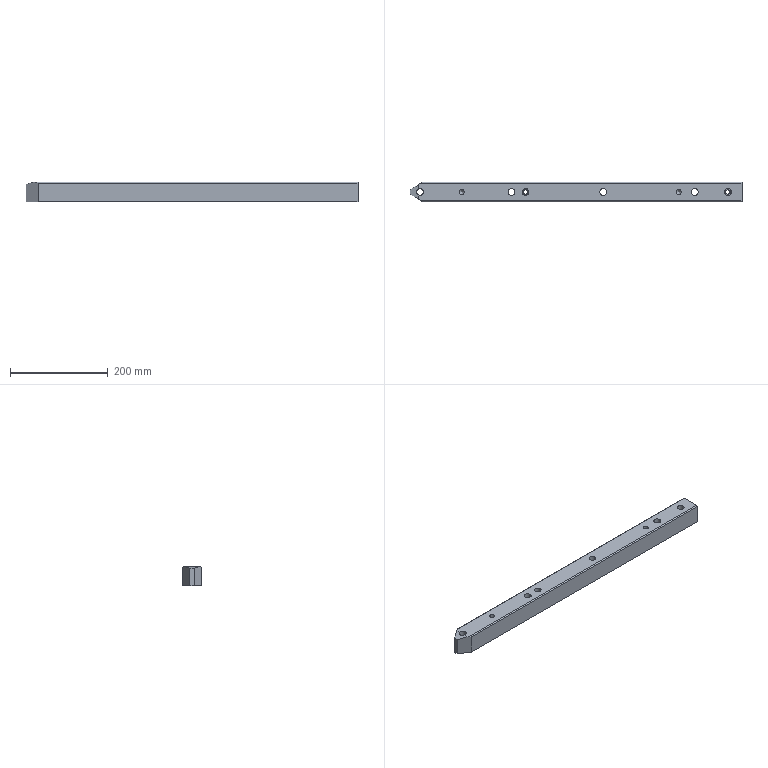Part | NX | features 22 2 | 1 solid | 35 faces | box 681 x 40 x 40 mm | volume 1019964 mm3 | plane 17 | cylinder 16 | cone 2 | commonest cylinder face diameters 14 x6 6 x4 9 x2 10.3 x2 25 x2
STEP:
#1=CARTESIAN_POINT('',(1685.15,0.,-3.5));
#2=VERTEX_POINT('',#1);
#3=CARTESIAN_POINT('',(1680.,0.,-3.5));
#4=DIRECTION('',(0.,0.,-1.));
#5=DIRECTION('',(1.,0.,0.));
#6=AXIS2_PLACEMENT_3D('',#3,#4,#5);
#7=CIRCLE('',#6,5.15);
#8=EDGE_CURVE('',#2,#2,#7,.T.);
#9=ORIENTED_EDGE('',*,*,#8,.T.);
#10=EDGE_LOOP('',(#9));
#11=FACE_BOUND('',#10,.T.);
#12=CARTESIAN_POINT('',(1344.306,0.,-3.5));
#13=VERTEX_POINT('',#12);
#14=CARTESIAN_POINT('',(1337.306,0.,-3.5));
#15=DIRECTION('',(0.,0.,-1.));
#16=DIRECTION('',(1.,0.,0.));
#17=AXIS2_PLACEMENT_3D('',#14,#15,#16);
#18=CIRCLE('',#17,7.);
#19=EDGE_CURVE('',#13,#13,#18,.T.);
#20=ORIENTED_EDGE('',*,*,#19,.T.);
#21=EDGE_LOOP('',(#20));
#22=FACE_BOUND('',#21,.T.);
#23=CARTESIAN_POINT('',(1372.578,2.394,-3.5));
#24=VERTEX_POINT('',#23);
#25=CARTESIAN_POINT('',(1366.,0.,-3.5));
#26=DIRECTION('',(0.,0.,-1.));
#27=DIRECTION('',(0.9397,0.342,0.));
#28=AXIS2_PLACEMENT_3D('',#25,#26,#27);
#29=CIRCLE('',#28,7.);
#30=EDGE_CURVE('',#24,#24,#29,.T.);
#31=ORIENTED_EDGE('',*,*,#30,.T.);
#32=EDGE_LOOP('',(#31));
#33=FACE_BOUND('',#32,.T.);
#34=CARTESIAN_POINT('',(1787.578,2.394,-3.5));
#35=VERTEX_POINT('',#34);
#36=CARTESIAN_POINT('',(1781.,0.,-3.5));
#37=DIRECTION('',(0.,0.,-1.));
#38=DIRECTION('',(0.9397,0.342,0.));
#39=AXIS2_PLACEMENT_3D('',#36,#37,#38);
#40=CIRCLE('',#39,7.);
#41=EDGE_CURVE('',#35,#35,#40,.T.);
#42=ORIENTED_EDGE('',*,*,#41,.T.);
#43=EDGE_LOOP('',(#42));
#44=FACE_BOUND('',#43,.T.);
#45=CARTESIAN_POINT('',(1146.,6.17,-3.5));
#46=VERTEX_POINT('',#45);
#47=CARTESIAN_POINT('',(1146.,-6.17,-3.5));
#48=VERTEX_POINT('',#47);
#49=CARTESIAN_POINT('',(1149.306,0.,-3.5));
#50=DIRECTION('',(0.,0.,-1.));
#51=DIRECTION('',(1.,0.,0.));
#52=AXIS2_PLACEMENT_3D('',#49,#50,#51);
#53=CIRCLE('',#52,7.);
#54=EDGE_CURVE('',#46,#48,#53,.T.);
#55=ORIENTED_EDGE('',*,*,#54,.T.);
#56=CARTESIAN_POINT('',(1146.,-14.83,-3.5));
#57=VERTEX_POINT('',#56);
#58=CARTESIAN_POINT('',(1146.,0.,-3.5));
#59=DIRECTION('',(0.,-1.,0.));
#60=VECTOR('',#59,1000.);
#61=LINE('',#58,#60);
#62=EDGE_CURVE('',#48,#57,#61,.T.);
#63=ORIENTED_EDGE('',*,*,#62,.T.);
#64=CARTESIAN_POINT('',(1151.084,-18.,-3.5));
#65=VERTEX_POINT('',#64);
#66=CARTESIAN_POINT('',(921.823,124.98,-3.5));
#67=DIRECTION('',(0.8485,-0.5292,0.));
#68=VECTOR('',#67,1000.);
#69=LINE('',#66,#68);
#70=EDGE_CURVE('',#57,#65,#69,.T.);
#71=ORIENTED_EDGE('',*,*,#70,.T.);
#72=CARTESIAN_POINT('',(1810.,-18.,-3.5));
#73=VERTEX_POINT('',#72);
#74=CARTESIAN_POINT('',(883.879,-18.,-3.5));
#75=DIRECTION('',(1.,0.,0.));
#76=VECTOR('',#75,1000.);
#77=LINE('',#74,#76);
#78=EDGE_CURVE('',#65,#73,#77,.T.);
#79=ORIENTED_EDGE('',*,*,#78,.T.);
#80=CARTESIAN_POINT('',(1810.,18.,-3.5));
#81=VERTEX_POINT('',#80);
#82=CARTESIAN_POINT('',(1810.,0.,-3.5));
#83=DIRECTION('',(0.,1.,0.));
#84=VECTOR('',#83,1000.);
#85=LINE('',#82,#84);
#86=EDGE_CURVE('',#73,#81,#85,.T.);
#87=ORIENTED_EDGE('',*,*,#86,.T.);
#88=CARTESIAN_POINT('',(1151.084,18.,-3.5));
#89=VERTEX_POINT('',#88);
#90=CARTESIAN_POINT('',(883.879,18.,-3.5));
#91=DIRECTION('',(-1.,0.,0.));
#92=VECTOR('',#91,1000.);
#93=LINE('',#90,#92);
#94=EDGE_CURVE('',#81,#89,#93,.T.);
#95=ORIENTED_EDGE('',*,*,#94,.T.);
#96=CARTESIAN_POINT('',(1146.,14.83,-3.5));
#97=VERTEX_POINT('',#96);
#98=CARTESIAN_POINT('',(1130.298,5.037,-3.5));
#99=DIRECTION('',(0.8485,0.5292,0.));
#100=VECTOR('',#99,1000.);
#101=LINE('',#98,#100);
#102=EDGE_CURVE('',#97,#89,#101,.T.);
#103=ORIENTED_EDGE('',*,*,#102,.F.);
#104=CARTESIAN_POINT('',(1146.,0.,-3.5));
#105=DIRECTION('',(0.,-1.,0.));
#106=VECTOR('',#105,1000.);
#107=LINE('',#104,#106);
#108=EDGE_CURVE('',#97,#46,#107,.T.);
#109=ORIENTED_EDGE('',*,*,#108,.T.);
#110=EDGE_LOOP('',(#55,#63,#71,#79,#87,#95,#103,#109));
#111=FACE_BOUND('',#110,.T.);
#112=CARTESIAN_POINT('',(1532.306,0.,-3.5));
#113=VERTEX_POINT('',#112);
#114=CARTESIAN_POINT('',(1525.306,0.,-3.5));
#115=DIRECTION('',(0.,0.,1.));
#116=DIRECTION('',(1.,0.,0.));
#117=AXIS2_PLACEMENT_3D('',#114,#115,#116);
#118=CIRCLE('',#117,7.);
#119=EDGE_CURVE('',#113,#113,#118,.T.);
#120=ORIENTED_EDGE('',*,*,#119,.F.);
#121=EDGE_LOOP('',(#120));
#122=FACE_BOUND('',#121,.T.);
#123=CARTESIAN_POINT('',(1720.306,0.,-3.5));
#124=VERTEX_POINT('',#123);
#125=CARTESIAN_POINT('',(1713.306,0.,-3.5));
#126=DIRECTION('',(0.,0.,1.));
#127=DIRECTION('',(1.,0.,0.));
#128=AXIS2_PLACEMENT_3D('',#125,#126,#127);
#129=CIRCLE('',#128,7.);
#130=EDGE_CURVE('',#124,#124,#129,.T.);
#131=ORIENTED_EDGE('',*,*,#130,.F.);
#132=EDGE_LOOP('',(#131));
#133=FACE_BOUND('',#132,.T.);
#134=CARTESIAN_POINT('',(1240.15,0.,-3.5));
#135=VERTEX_POINT('',#134);
#136=CARTESIAN_POINT('',(1235.,0.,-3.5));
#137=DIRECTION('',(0.,0.,-1.));
#138=DIRECTION('',(1.,0.,0.));
#139=AXIS2_PLACEMENT_3D('',#136,#137,#138);
#140=CIRCLE('',#139,5.15);
#141=EDGE_CURVE('',#135,#135,#140,.T.);
#142=ORIENTED_EDGE('',*,*,#141,.T.);
#143=EDGE_LOOP('',(#142));
#144=FACE_BOUND('',#143,.T.);
#145=CARTESIAN_POINT('',(883.879,0.,-3.5));
#146=DIRECTION('',(0.,0.,1.));
#147=DIRECTION('',(-1.,0.,0.));
#148=AXIS2_PLACEMENT_3D('',#145,#146,#147);
#149=PLANE('',#148);
#150=ADVANCED_FACE('',(#11,#22,#33,#44,#111,#122,#133,#144),#149,.T.);
#151=CARTESIAN_POINT('',(1344.306,0.,-43.5));
#152=VERTEX_POINT('',#151);
#153=CARTESIAN_POINT('',(1337.306,0.,-43.5));
#154=DIRECTION('',(0.,0.,-1.));
#155=DIRECTION('',(1.,0.,0.));
#156=AXIS2_PLACEMENT_3D('',#153,#154,#155);
#157=CIRCLE('',#156,7.);
#158=EDGE_CURVE('',#152,#152,#157,.T.);
#159=ORIENTED_EDGE('',*,*,#158,.F.);
#160=EDGE_LOOP('',(#159));
#161=FACE_BOUND('',#160,.T.);
#162=CARTESIAN_POINT('',(1810.,20.,-43.5));
#163=VERTEX_POINT('',#162);
#164=CARTESIAN_POINT('',(1154.291,20.,-43.5));
#165=VERTEX_POINT('',#164);
#166=CARTESIAN_POINT('',(1199.,20.,-43.5));
#167=DIRECTION('',(-1.,0.,0.));
#168=VECTOR('',#167,1000.);
#169=LINE('',#166,#168);
#170=EDGE_CURVE('',#163,#165,#169,.T.);
#171=ORIENTED_EDGE('',*,*,#170,.F.);
#172=CARTESIAN_POINT('',(1810.,-20.,-43.5));
#173=VERTEX_POINT('',#172);
#174=CARTESIAN_POINT('',(1810.,0.,-43.5));
#175=DIRECTION('',(0.,-1.,0.));
#176=VECTOR('',#175,1000.);
#177=LINE('',#174,#176);
#178=EDGE_CURVE('',#163,#173,#177,.T.);
#179=ORIENTED_EDGE('',*,*,#178,.T.);
#180=CARTESIAN_POINT('',(1154.291,-20.,-43.5));
#181=VERTEX_POINT('',#180);
#182=CARTESIAN_POINT('',(1199.,-20.,-43.5));
#183=DIRECTION('',(1.,0.,0.));
#184=VECTOR('',#183,1000.);
#185=LINE('',#182,#184);
#186=EDGE_CURVE('',#181,#173,#185,.T.);
#187=ORIENTED_EDGE('',*,*,#186,.F.);
#188=CARTESIAN_POINT('',(1129.,-4.227,-43.5));
#189=VERTEX_POINT('',#188);
#190=CARTESIAN_POINT('',(921.823,124.98,-43.5));
#191=DIRECTION('',(-0.8485,0.5292,0.));
#192=VECTOR('',#191,1000.);
#193=LINE('',#190,#192);
#194=EDGE_CURVE('',#181,#189,#193,.T.);
#195=ORIENTED_EDGE('',*,*,#194,.T.);
#196=CARTESIAN_POINT('',(1129.,4.227,-43.5));
#197=VERTEX_POINT('',#196);
#198=CARTESIAN_POINT('',(1129.,0.,-43.5));
#199=DIRECTION('',(0.,-1.,0.));
#200=VECTOR('',#199,1000.);
#201=LINE('',#198,#200);
#202=EDGE_CURVE('',#197,#189,#201,.T.);
#203=ORIENTED_EDGE('',*,*,#202,.F.);
#204=CARTESIAN_POINT('',(921.823,-124.98,-43.5));
#205=DIRECTION('',(0.8485,0.5292,0.));
#206=VECTOR('',#205,1000.);
#207=LINE('',#204,#206);
#208=EDGE_CURVE('',#197,#165,#207,.T.);
#209=ORIENTED_EDGE('',*,*,#208,.T.);
#210=EDGE_LOOP('',(#171,#179,#187,#195,#203,#209));
#211=FACE_BOUND('',#210,.T.);
#212=CARTESIAN_POINT('',(1783.701,-11.,-43.5));
#213=VERTEX_POINT('',#212);
#214=CARTESIAN_POINT('',(1778.299,-11.,-43.5));
#215=VERTEX_POINT('',#214);
#216=CARTESIAN_POINT('',(1781.,-11.,-43.5));
#217=DIRECTION('',(-1.,0.,0.));
#218=VECTOR('',#217,1000.);
#219=LINE('',#216,#218);
#220=EDGE_CURVE('',#213,#215,#219,.T.);
#221=ORIENTED_EDGE('',*,*,#220,.F.);
#222=CARTESIAN_POINT('',(1788.847,-9.73,-43.5));
#223=VERTEX_POINT('',#222);
#224=CARTESIAN_POINT('',(1785.937,-9.,-43.5));
#225=DIRECTION('',(0.,0.,-1.));
#226=DIRECTION('',(1.,0.,0.));
#227=AXIS2_PLACEMENT_3D('',#224,#225,#226);
#228=CIRCLE('',#227,3.);
#229=EDGE_CURVE('',#223,#213,#228,.T.);
#230=ORIENTED_EDGE('',*,*,#229,.F.);
#231=CARTESIAN_POINT('',(1773.153,-9.73,-43.5));
#232=VERTEX_POINT('',#231);
#233=CARTESIAN_POINT('',(1781.,0.,-43.5));
#234=DIRECTION('',(0.,0.,-1.));
#235=DIRECTION('',(1.,0.,0.));
#236=AXIS2_PLACEMENT_3D('',#233,#234,#235);
#237=CIRCLE('',#236,12.5);
#238=EDGE_CURVE('',#232,#223,#237,.T.);
#239=ORIENTED_EDGE('',*,*,#238,.F.);
#240=CARTESIAN_POINT('',(1776.063,-9.,-43.5));
#241=DIRECTION('',(0.,0.,-1.));
#242=DIRECTION('',(1.,0.,0.));
#243=AXIS2_PLACEMENT_3D('',#240,#241,#242);
#244=CIRCLE('',#243,3.);
#245=EDGE_CURVE('',#215,#232,#244,.T.);
#246=ORIENTED_EDGE('',*,*,#245,.F.);
#247=EDGE_LOOP('',(#221,#230,#239,#246));
#248=FACE_BOUND('',#247,.T.);
#249=CARTESIAN_POINT('',(1368.701,-11.,-43.5));
#250=VERTEX_POINT('',#249);
#251=CARTESIAN_POINT('',(1363.299,-11.,-43.5));
#252=VERTEX_POINT('',#251);
#253=CARTESIAN_POINT('',(1366.,-11.,-43.5));
#254=DIRECTION('',(-1.,0.,0.));
#255=VECTOR('',#254,1000.);
#256=LINE('',#253,#255);
#257=EDGE_CURVE('',#250,#252,#256,.T.);
#258=ORIENTED_EDGE('',*,*,#257,.F.);
#259=CARTESIAN_POINT('',(1373.847,-9.73,-43.5));
#260=VERTEX_POINT('',#259);
#261=CARTESIAN_POINT('',(1370.937,-9.,-43.5));
#262=DIRECTION('',(0.,0.,-1.));
#263=DIRECTION('',(0.9659,0.2588,0.));
#264=AXIS2_PLACEMENT_3D('',#261,#262,#263);
#265=CIRCLE('',#264,3.);
#266=EDGE_CURVE('',#260,#250,#265,.T.);
#267=ORIENTED_EDGE('',*,*,#266,.F.);
#268=CARTESIAN_POINT('',(1358.153,-9.73,-43.5));
#269=VERTEX_POINT('',#268);
#270=CARTESIAN_POINT('',(1366.,0.,-43.5));
#271=DIRECTION('',(0.,0.,1.));
#272=DIRECTION('',(0.9659,0.2588,0.));
#273=AXIS2_PLACEMENT_3D('',#270,#271,#272);
#274=CIRCLE('',#273,12.5);
#275=EDGE_CURVE('',#260,#269,#274,.T.);
#276=ORIENTED_EDGE('',*,*,#275,.T.);
#277=CARTESIAN_POINT('',(1361.063,-9.,-43.5));
#278=DIRECTION('',(0.,0.,-1.));
#279=DIRECTION('',(0.9659,0.2588,0.));
#280=AXIS2_PLACEMENT_3D('',#277,#278,#279);
#281=CIRCLE('',#280,3.);
#282=EDGE_CURVE('',#252,#269,#281,.T.);
#283=ORIENTED_EDGE('',*,*,#282,.F.);
#284=EDGE_LOOP('',(#258,#267,#276,#283));
#285=FACE_BOUND('',#284,.T.);
#286=CARTESIAN_POINT('',(1156.306,0.,-43.5));
#287=VERTEX_POINT('',#286);
#288=CARTESIAN_POINT('',(1149.306,0.,-43.5));
#289=DIRECTION('',(0.,0.,1.));
#290=DIRECTION('',(1.,0.,0.));
#291=AXIS2_PLACEMENT_3D('',#288,#289,#290);
#292=CIRCLE('',#291,7.);
#293=EDGE_CURVE('',#287,#287,#292,.T.);
#294=ORIENTED_EDGE('',*,*,#293,.T.);
#295=EDGE_LOOP('',(#294));
#296=FACE_BOUND('',#295,.T.);
#297=CARTESIAN_POINT('',(1532.306,0.,-43.5));
#298=VERTEX_POINT('',#297);
#299=CARTESIAN_POINT('',(1525.306,0.,-43.5));
#300=DIRECTION('',(0.,0.,1.));
#301=DIRECTION('',(1.,0.,0.));
#302=AXIS2_PLACEMENT_3D('',#299,#300,#301);
#303=CIRCLE('',#302,7.);
#304=EDGE_CURVE('',#298,#298,#303,.T.);
#305=ORIENTED_EDGE('',*,*,#304,.T.);
#306=EDGE_LOOP('',(#305));
#307=FACE_BOUND('',#306,.T.);
#308=CARTESIAN_POINT('',(1720.306,0.,-43.5));
#309=VERTEX_POINT('',#308);
#310=CARTESIAN_POINT('',(1713.306,0.,-43.5));
#311=DIRECTION('',(0.,0.,-1.));
#312=DIRECTION('',(1.,0.,0.));
#313=AXIS2_PLACEMENT_3D('',#310,#311,#312);
#314=CIRCLE('',#313,7.);
#315=EDGE_CURVE('',#309,#309,#314,.T.);
#316=ORIENTED_EDGE('',*,*,#315,.F.);
#317=EDGE_LOOP('',(#316));
#318=FACE_BOUND('',#317,.T.);
#319=CARTESIAN_POINT('',(883.879,0.,-43.5));
#320=DIRECTION('',(0.,0.,1.));
#321=DIRECTION('',(-1.,0.,0.));
#322=AXIS2_PLACEMENT_3D('',#319,#320,#321);
#323=PLANE('',#322);
#324=ADVANCED_FACE('',(#161,#211,#248,#285,#296,#307,#318),#323,.F.);
#325=CARTESIAN_POINT('',(1154.291,20.,-5.5));
#326=VERTEX_POINT('',#325);
#327=CARTESIAN_POINT('',(1810.,20.,-5.5));
#328=VERTEX_POINT('',#327);
#329=CARTESIAN_POINT('',(1199.,20.,-5.5));
#330=DIRECTION('',(1.,0.,0.));
#331=VECTOR('',#330,1000.);
#332=LINE('',#329,#331);
#333=EDGE_CURVE('',#326,#328,#332,.T.);
#334=ORIENTED_EDGE('',*,*,#333,.T.);
#335=CARTESIAN_POINT('',(1810.,20.,-23.5));
#336=DIRECTION('',(0.,0.,-1.));
#337=VECTOR('',#336,1000.);
#338=LINE('',#335,#337);
#339=EDGE_CURVE('',#328,#163,#338,.T.);
#340=ORIENTED_EDGE('',*,*,#339,.T.);
#341=ORIENTED_EDGE('',*,*,#170,.T.);
#342=CARTESIAN_POINT('',(1154.291,20.,-23.5));
#343=DIRECTION('',(0.,0.,1.));
#344=VECTOR('',#343,1000.);
#345=LINE('',#342,#344);
#346=EDGE_CURVE('',#165,#326,#345,.T.);
#347=ORIENTED_EDGE('',*,*,#346,.T.);
#348=EDGE_LOOP('',(#334,#340,#341,#347));
#349=FACE_BOUND('',#348,.T.);
#350=CARTESIAN_POINT('',(1199.,20.,-23.5));
#351=DIRECTION('',(0.,1.,0.));
#352=DIRECTION('',(0.,0.,-1.));
#353=AXIS2_PLACEMENT_3D('',#350,#351,#352);
#354=PLANE('',#353);
#355=ADVANCED_FACE('',(#349),#354,.T.);
#356=ORIENTED_EDGE('',*,*,#94,.F.);
#357=CARTESIAN_POINT('',(1810.,18.,-3.5));
#358=DIRECTION('',(0.,0.7071,-0.7071));
#359=VECTOR('',#358,1000.);
#360=LINE('',#357,#359);
#361=EDGE_CURVE('',#81,#328,#360,.T.);
#362=ORIENTED_EDGE('',*,*,#361,.T.);
#363=ORIENTED_EDGE('',*,*,#333,.F.);
#364=CARTESIAN_POINT('',(978.292,-89.762,104.262));
#365=DIRECTION('',(-0.75,-0.4677,0.4677));
#366=VECTOR('',#365,1000.);
#367=LINE('',#364,#366);
#368=EDGE_CURVE('',#326,#89,#367,.T.);
#369=ORIENTED_EDGE('',*,*,#368,.T.);
#370=EDGE_LOOP('',(#356,#362,#363,#369));
#371=FACE_BOUND('',#370,.T.);
#372=CARTESIAN_POINT('',(883.879,18.,-3.5));
#373=DIRECTION('',(0.,-0.7071,-0.7071));
#374=DIRECTION('',(0.,-0.7071,0.7071));
#375=AXIS2_PLACEMENT_3D('',#372,#373,#374);
#376=PLANE('',#375);
#377=ADVANCED_FACE('',(#371),#376,.F.);
#378=ORIENTED_EDGE('',*,*,#186,.T.);
#379=CARTESIAN_POINT('',(1810.,-20.,-5.5));
#380=VERTEX_POINT('',#379);
#381=CARTESIAN_POINT('',(1810.,-20.,-23.5));
#382=DIRECTION('',(0.,0.,1.));
#383=VECTOR('',#382,1000.);
#384=LINE('',#381,#383);
#385=EDGE_CURVE('',#173,#380,#384,.T.);
#386=ORIENTED_EDGE('',*,*,#385,.T.);
#387=CARTESIAN_POINT('',(1154.291,-20.,-5.5));
#388=VERTEX_POINT('',#387);
#389=CARTESIAN_POINT('',(1199.,-20.,-5.5));
#390=DIRECTION('',(-1.,0.,0.));
#391=VECTOR('',#390,1000.);
#392=LINE('',#389,#391);
#393=EDGE_CURVE('',#380,#388,#392,.T.);
#394=ORIENTED_EDGE('',*,*,#393,.T.);
#395=CARTESIAN_POINT('',(1154.291,-20.,-23.5));
#396=DIRECTION('',(0.,0.,-1.));
#397=VECTOR('',#396,1000.);
#398=LINE('',#395,#397);
#399=EDGE_CURVE('',#388,#181,#398,.T.);
#400=ORIENTED_EDGE('',*,*,#399,.T.);
#401=EDGE_LOOP('',(#378,#386,#394,#400));
#402=FACE_BOUND('',#401,.T.);
#403=CARTESIAN_POINT('',(1199.,-20.,-23.5));
#404=DIRECTION('',(0.,-1.,0.));
#405=DIRECTION('',(0.,0.,1.));
#406=AXIS2_PLACEMENT_3D('',#403,#404,#405);
#407=PLANE('',#406);
#408=ADVANCED_FACE('',(#402),#407,.T.);
#409=ORIENTED_EDGE('',*,*,#393,.F.);
#410=CARTESIAN_POINT('',(1810.,-18.,-3.5));
#411=DIRECTION('',(0.,0.7071,0.7071));
#412=VECTOR('',#411,1000.);
#413=LINE('',#410,#412);
#414=EDGE_CURVE('',#380,#73,#413,.T.);
#415=ORIENTED_EDGE('',*,*,#414,.T.);
#416=ORIENTED_EDGE('',*,*,#78,.F.);
#417=CARTESIAN_POINT('',(978.292,89.762,104.262));
#418=DIRECTION('',(0.75,-0.4677,-0.4677));
#419=VECTOR('',#418,1000.);
#420=LINE('',#417,#419);
#421=EDGE_CURVE('',#65,#388,#420,.T.);
#422=ORIENTED_EDGE('',*,*,#421,.T.);
#423=EDGE_LOOP('',(#409,#415,#416,#422));
#424=FACE_BOUND('',#423,.T.);
#425=CARTESIAN_POINT('',(883.879,-18.,-3.5));
#426=DIRECTION('',(0.,0.7071,-0.7071));
#427=DIRECTION('',(0.,-0.7071,-0.7071));
#428=AXIS2_PLACEMENT_3D('',#425,#426,#427);
#429=PLANE('',#428);
#430=ADVANCED_FACE('',(#424),#429,.F.);
#431=CARTESIAN_POINT('',(1129.,-4.227,-7.75));
#432=VERTEX_POINT('',#431);
#433=CARTESIAN_POINT('',(1124.987,-1.725,-8.753));
#434=DIRECTION('',(0.83,-0.5177,0.2075));
#435=VECTOR('',#434,1000.);
#436=LINE('',#433,#435);
#437=EDGE_CURVE('',#432,#57,#436,.T.);
#438=ORIENTED_EDGE('',*,*,#437,.F.);
#439=CARTESIAN_POINT('',(1129.,-4.227,-23.5));
#440=DIRECTION('',(0.,0.,1.));
#441=VECTOR('',#440,1000.);
#442=LINE('',#439,#441);
#443=EDGE_CURVE('',#189,#432,#442,.T.);
#444=ORIENTED_EDGE('',*,*,#443,.F.);
#445=ORIENTED_EDGE('',*,*,#194,.F.);
#446=ORIENTED_EDGE('',*,*,#399,.F.);
#447=ORIENTED_EDGE('',*,*,#421,.F.);
#448=ORIENTED_EDGE('',*,*,#70,.F.);
#449=EDGE_LOOP('',(#438,#444,#445,#446,#447,#448));
#450=FACE_BOUND('',#449,.T.);
#451=CARTESIAN_POINT('',(1130.298,-5.037,-13.5));
#452=DIRECTION('',(-0.5292,-0.8485,0.));
#453=DIRECTION('',(0.8485,-0.5292,0.));
#454=AXIS2_PLACEMENT_3D('',#451,#452,#453);
#455=PLANE('',#454);
#456=ADVANCED_FACE('',(#450),#455,.T.);
#457=CARTESIAN_POINT('',(1781.,-4.5,-28.5));
#458=VERTEX_POINT('',#457);
#459=CARTESIAN_POINT('',(1781.,0.,-28.5));
#460=DIRECTION('',(0.,0.,1.));
#461=DIRECTION('',(0.,-1.,0.));
#462=AXIS2_PLACEMENT_3D('',#459,#460,#461);
#463=CIRCLE('',#462,4.5);
#464=EDGE_CURVE('',#458,#458,#463,.T.);
#465=ORIENTED_EDGE('',*,*,#464,.F.);
#466=EDGE_LOOP('',(#465));
#467=FACE_BOUND('',#466,.T.);
#468=CARTESIAN_POINT('',(1781.,-4.5,-15.5));
#469=VERTEX_POINT('',#468);
#470=CARTESIAN_POINT('',(1781.,0.,-15.5));
#471=DIRECTION('',(0.,0.,1.));
#472=DIRECTION('',(0.,-1.,0.));
#473=AXIS2_PLACEMENT_3D('',#470,#471,#472);
#474=CIRCLE('',#473,4.5);
#475=EDGE_CURVE('',#469,#469,#474,.T.);
#476=ORIENTED_EDGE('',*,*,#475,.T.);
#477=EDGE_LOOP('',(#476));
#478=FACE_BOUND('',#477,.T.);
#479=CARTESIAN_POINT('',(1781.,0.,49.9));
#480=DIRECTION('',(0.,0.,-1.));
#481=DIRECTION('',(0.342,-0.9397,0.));
#482=AXIS2_PLACEMENT_3D('',#479,#480,#481);
#483=CYLINDRICAL_SURFACE('',#482,4.5);
#484=ADVANCED_FACE('',(#467,#478),#483,.F.);
#485=CARTESIAN_POINT('',(1370.229,1.539,-28.5));
#486=VERTEX_POINT('',#485);
#487=CARTESIAN_POINT('',(1366.,0.,-28.5));
#488=DIRECTION('',(0.,0.,1.));
#489=DIRECTION('',(0.9397,0.342,0.));
#490=AXIS2_PLACEMENT_3D('',#487,#488,#489);
#491=CIRCLE('',#490,4.5);
#492=EDGE_CURVE('',#486,#486,#491,.T.);
#493=ORIENTED_EDGE('',*,*,#492,.F.);
#494=EDGE_LOOP('',(#493));
#495=FACE_BOUND('',#494,.T.);
#496=CARTESIAN_POINT('',(1370.5,0.,-15.5));
#497=VERTEX_POINT('',#496);
#498=CARTESIAN_POINT('',(1366.,0.,-15.5));
#499=DIRECTION('',(0.,0.,1.));
#500=DIRECTION('',(1.,0.,0.));
#501=AXIS2_PLACEMENT_3D('',#498,#499,#500);
#502=CIRCLE('',#501,4.5);
#503=EDGE_CURVE('',#497,#497,#502,.T.);
#504=ORIENTED_EDGE('',*,*,#503,.T.);
#505=EDGE_LOOP('',(#504));
#506=FACE_BOUND('',#505,.T.);
#507=CARTESIAN_POINT('',(1366.,0.,49.9));
#508=DIRECTION('',(0.,0.,-1.));
#509=DIRECTION('',(0.342,-0.9397,0.));
#510=AXIS2_PLACEMENT_3D('',#507,#508,#509);
#511=CYLINDRICAL_SURFACE('',#510,4.5);
#512=ADVANCED_FACE('',(#495,#506),#511,.F.);
#513=ORIENTED_EDGE('',*,*,#492,.T.);
#514=EDGE_LOOP('',(#513));
#515=FACE_BOUND('',#514,.T.);
#516=CARTESIAN_POINT('',(1363.299,-11.,-28.5));
#517=VERTEX_POINT('',#516);
#518=CARTESIAN_POINT('',(1358.153,-9.73,-28.5));
#519=VERTEX_POINT('',#518);
#520=CARTESIAN_POINT('',(1361.063,-9.,-28.5));
#521=DIRECTION('',(0.,0.,-1.));
#522=DIRECTION('',(0.9397,-0.342,0.));
#523=AXIS2_PLACEMENT_3D('',#520,#521,#522);
#524=CIRCLE('',#523,3.);
#525=EDGE_CURVE('',#517,#519,#524,.T.);
#526=ORIENTED_EDGE('',*,*,#525,.T.);
#527=CARTESIAN_POINT('',(1373.847,-9.73,-28.5));
#528=VERTEX_POINT('',#527);
#529=CARTESIAN_POINT('',(1366.,0.,-28.5));
#530=DIRECTION('',(0.,0.,-1.));
#531=DIRECTION('',(0.,1.,0.));
#532=AXIS2_PLACEMENT_3D('',#529,#530,#531);
#533=CIRCLE('',#532,12.5);
#534=EDGE_CURVE('',#519,#528,#533,.T.);
#535=ORIENTED_EDGE('',*,*,#534,.T.);
#536=CARTESIAN_POINT('',(1368.701,-11.,-28.5));
#537=VERTEX_POINT('',#536);
#538=CARTESIAN_POINT('',(1370.937,-9.,-28.5));
#539=DIRECTION('',(0.,0.,1.));
#540=DIRECTION('',(-0.9397,-0.342,0.));
#541=AXIS2_PLACEMENT_3D('',#538,#539,#540);
#542=CIRCLE('',#541,3.);
#543=EDGE_CURVE('',#537,#528,#542,.T.);
#544=ORIENTED_EDGE('',*,*,#543,.F.);
#545=CARTESIAN_POINT('',(1366.,-11.,-28.5));
#546=DIRECTION('',(-1.,0.,0.));
#547=VECTOR('',#546,1000.);
#548=LINE('',#545,#547);
#549=EDGE_CURVE('',#537,#517,#548,.T.);
#550=ORIENTED_EDGE('',*,*,#549,.T.);
#551=EDGE_LOOP('',(#526,#535,#544,#550));
#552=FACE_BOUND('',#551,.T.);
#553=CARTESIAN_POINT('',(1366.,0.,-28.5));
#554=DIRECTION('',(0.,0.,1.));
#555=DIRECTION('',(0.,-1.,0.));
#556=AXIS2_PLACEMENT_3D('',#553,#554,#555);
#557=PLANE('',#556);
#558=ADVANCED_FACE('',(#515,#552),#557,.F.);
#559=ORIENTED_EDGE('',*,*,#464,.T.);
#560=EDGE_LOOP('',(#559));
#561=FACE_BOUND('',#560,.T.);
#562=CARTESIAN_POINT('',(1778.299,-11.,-28.5));
#563=VERTEX_POINT('',#562);
#564=CARTESIAN_POINT('',(1773.153,-9.73,-28.5));
#565=VERTEX_POINT('',#564);
#566=CARTESIAN_POINT('',(1776.063,-9.,-28.5));
#567=DIRECTION('',(0.,0.,-1.));
#568=DIRECTION('',(0.,-1.,0.));
#569=AXIS2_PLACEMENT_3D('',#566,#567,#568);
#570=CIRCLE('',#569,3.);
#571=EDGE_CURVE('',#563,#565,#570,.T.);
#572=ORIENTED_EDGE('',*,*,#571,.T.);
#573=CARTESIAN_POINT('',(1788.847,-9.73,-28.5));
#574=VERTEX_POINT('',#573);
#575=CARTESIAN_POINT('',(1781.,0.,-28.5));
#576=DIRECTION('',(0.,0.,-1.));
#577=DIRECTION('',(0.,-1.,0.));
#578=AXIS2_PLACEMENT_3D('',#575,#576,#577);
#579=CIRCLE('',#578,12.5);
#580=EDGE_CURVE('',#565,#574,#579,.T.);
#581=ORIENTED_EDGE('',*,*,#580,.T.);
#582=CARTESIAN_POINT('',(1783.701,-11.,-28.5));
#583=VERTEX_POINT('',#582);
#584=CARTESIAN_POINT('',(1785.937,-9.,-28.5));
#585=DIRECTION('',(0.,0.,1.));
#586=DIRECTION('',(0.,-1.,0.));
#587=AXIS2_PLACEMENT_3D('',#584,#585,#586);
#588=CIRCLE('',#587,3.);
#589=EDGE_CURVE('',#583,#574,#588,.T.);
#590=ORIENTED_EDGE('',*,*,#589,.F.);
#591=CARTESIAN_POINT('',(1781.,-11.,-28.5));
#592=DIRECTION('',(-1.,0.,0.));
#593=VECTOR('',#592,1000.);
#594=LINE('',#591,#593);
#595=EDGE_CURVE('',#583,#563,#594,.T.);
#596=ORIENTED_EDGE('',*,*,#595,.T.);
#597=EDGE_LOOP('',(#572,#581,#590,#596));
#598=FACE_BOUND('',#597,.T.);
#599=CARTESIAN_POINT('',(1781.,0.,-28.5));
#600=DIRECTION('',(0.,0.,1.));
#601=DIRECTION('',(0.,-1.,0.));
#602=AXIS2_PLACEMENT_3D('',#599,#600,#601);
#603=PLANE('',#602);
#604=ADVANCED_FACE('',(#561,#598),#603,.F.);
#605=CARTESIAN_POINT('',(1781.,-7.,-15.5));
#606=VERTEX_POINT('',#605);
#607=CARTESIAN_POINT('',(1781.,0.,-15.5));
#608=DIRECTION('',(0.,0.,1.));
#609=DIRECTION('',(0.,-1.,0.));
#610=AXIS2_PLACEMENT_3D('',#607,#608,#609);
#611=CIRCLE('',#610,7.);
#612=EDGE_CURVE('',#606,#606,#611,.T.);
#613=ORIENTED_EDGE('',*,*,#612,.T.);
#614=EDGE_LOOP('',(#613));
#615=FACE_BOUND('',#614,.T.);
#616=ORIENTED_EDGE('',*,*,#475,.F.);
#617=EDGE_LOOP('',(#616));
#618=FACE_BOUND('',#617,.T.);
#619=CARTESIAN_POINT('',(1889.182,268.173,-15.5));
#620=DIRECTION('',(0.,0.,1.));
#621=DIRECTION('',(-0.9397,-0.342,0.));
#622=AXIS2_PLACEMENT_3D('',#619,#620,#621);
#623=PLANE('',#622);
#624=ADVANCED_FACE('',(#615,#618),#623,.T.);
#625=CARTESIAN_POINT('',(1373.,0.,-15.5));
#626=VERTEX_POINT('',#625);
#627=CARTESIAN_POINT('',(1366.,0.,-15.5));
#628=DIRECTION('',(0.,0.,1.));
#629=DIRECTION('',(1.,0.,0.));
#630=AXIS2_PLACEMENT_3D('',#627,#628,#629);
#631=CIRCLE('',#630,7.);
#632=EDGE_CURVE('',#626,#626,#631,.T.);
#633=ORIENTED_EDGE('',*,*,#632,.T.);
#634=EDGE_LOOP('',(#633));
#635=FACE_BOUND('',#634,.T.);
#636=ORIENTED_EDGE('',*,*,#503,.F.);
#637=EDGE_LOOP('',(#636));
#638=FACE_BOUND('',#637,.T.);
#639=CARTESIAN_POINT('',(1474.182,268.173,-15.5));
#640=DIRECTION('',(0.,0.,1.));
#641=DIRECTION('',(-0.9397,-0.342,0.));
#642=AXIS2_PLACEMENT_3D('',#639,#640,#641);
#643=PLANE('',#642);
#644=ADVANCED_FACE('',(#635,#638),#643,.T.);
#645=CARTESIAN_POINT('',(1358.153,-9.73,-34.));
#646=DIRECTION('',(0.,0.,-1.));
#647=VECTOR('',#646,1000.);
#648=LINE('',#645,#647);
#649=EDGE_CURVE('',#519,#269,#648,.T.);
#650=ORIENTED_EDGE('',*,*,#649,.F.);
#651=ORIENTED_EDGE('',*,*,#525,.F.);
#652=CARTESIAN_POINT('',(1363.299,-11.,-41.5));
#653=DIRECTION('',(0.,0.,1.));
#654=VECTOR('',#653,1000.);
#655=LINE('',#652,#654);
#656=EDGE_CURVE('',#252,#517,#655,.T.);
#657=ORIENTED_EDGE('',*,*,#656,.F.);
#658=ORIENTED_EDGE('',*,*,#282,.T.);
#659=EDGE_LOOP('',(#650,#651,#657,#658));
#660=FACE_BOUND('',#659,.T.);
#661=CARTESIAN_POINT('',(1361.063,-9.,-41.5));
#662=DIRECTION('',(0.,0.,1.));
#663=DIRECTION('',(0.9397,-0.342,0.));
#664=AXIS2_PLACEMENT_3D('',#661,#662,#663);
#665=CYLINDRICAL_SURFACE('',#664,3.);
#666=ADVANCED_FACE('',(#660),#665,.F.);
#667=CARTESIAN_POINT('',(1373.847,-9.73,-34.));
#668=DIRECTION('',(0.,0.,-1.));
#669=VECTOR('',#668,1000.);
#670=LINE('',#667,#669);
#671=EDGE_CURVE('',#528,#260,#670,.T.);
#672=ORIENTED_EDGE('',*,*,#671,.F.);
#673=ORIENTED_EDGE('',*,*,#534,.F.);
#674=ORIENTED_EDGE('',*,*,#649,.T.);
#675=ORIENTED_EDGE('',*,*,#275,.F.);
#676=EDGE_LOOP('',(#672,#673,#674,#675));
#677=FACE_BOUND('',#676,.T.);
#678=CARTESIAN_POINT('',(1366.,0.,-96.5));
#679=DIRECTION('',(0.,0.,-1.));
#680=DIRECTION('',(0.,1.,0.));
#681=AXIS2_PLACEMENT_3D('',#678,#679,#680);
#682=CYLINDRICAL_SURFACE('',#681,12.5);
#683=ADVANCED_FACE('',(#677),#682,.F.);
#684=ORIENTED_EDGE('',*,*,#671,.T.);
#685=ORIENTED_EDGE('',*,*,#266,.T.);
#686=CARTESIAN_POINT('',(1368.701,-11.,-41.5));
#687=DIRECTION('',(0.,0.,1.));
#688=VECTOR('',#687,1000.);
#689=LINE('',#686,#688);
#690=EDGE_CURVE('',#250,#537,#689,.T.);
#691=ORIENTED_EDGE('',*,*,#690,.T.);
#692=ORIENTED_EDGE('',*,*,#543,.T.);
#693=EDGE_LOOP('',(#684,#685,#691,#692));
#694=FACE_BOUND('',#693,.T.);
#695=CARTESIAN_POINT('',(1370.937,-9.,-41.5));
#696=DIRECTION('',(0.,0.,1.));
#697=DIRECTION('',(-0.9397,-0.342,0.));
#698=AXIS2_PLACEMENT_3D('',#695,#696,#697);
#699=CYLINDRICAL_SURFACE('',#698,3.);
#700=ADVANCED_FACE('',(#694),#699,.F.);
#701=ORIENTED_EDGE('',*,*,#549,.F.);
#702=ORIENTED_EDGE('',*,*,#690,.F.);
#703=ORIENTED_EDGE('',*,*,#257,.T.);
#704=ORIENTED_EDGE('',*,*,#656,.T.);
#705=EDGE_LOOP('',(#701,#702,#703,#704));
#706=FACE_BOUND('',#705,.T.);
#707=CARTESIAN_POINT('',(1366.,-11.,-126.5));
#708=DIRECTION('',(0.,1.,0.));
#709=DIRECTION('',(0.,0.,-1.));
#710=AXIS2_PLACEMENT_3D('',#707,#708,#709);
#711=PLANE('',#710);
#712=ADVANCED_FACE('',(#706),#711,.T.);
#713=CARTESIAN_POINT('',(1773.153,-9.73,-34.));
#714=DIRECTION('',(0.,0.,-1.));
#715=VECTOR('',#714,1000.);
#716=LINE('',#713,#715);
#717=EDGE_CURVE('',#565,#232,#716,.T.);
#718=ORIENTED_EDGE('',*,*,#717,.F.);
#719=ORIENTED_EDGE('',*,*,#571,.F.);
#720=CARTESIAN_POINT('',(1778.299,-11.,-41.5));
#721=DIRECTION('',(0.,0.,1.));
#722=VECTOR('',#721,1000.);
#723=LINE('',#720,#722);
#724=EDGE_CURVE('',#215,#563,#723,.T.);
#725=ORIENTED_EDGE('',*,*,#724,.F.);
#726=ORIENTED_EDGE('',*,*,#245,.T.);
#727=EDGE_LOOP('',(#718,#719,#725,#726));
#728=FACE_BOUND('',#727,.T.);
#729=CARTESIAN_POINT('',(1776.063,-9.,-41.5));
#730=DIRECTION('',(0.,0.,1.));
#731=DIRECTION('',(0.9397,-0.342,0.));
#732=AXIS2_PLACEMENT_3D('',#729,#730,#731);
#733=CYLINDRICAL_SURFACE('',#732,3.);
#734=ADVANCED_FACE('',(#728),#733,.F.);
#735=CARTESIAN_POINT('',(1788.847,-9.73,-34.));
#736=DIRECTION('',(0.,0.,-1.));
#737=VECTOR('',#736,1000.);
#738=LINE('',#735,#737);
#739=EDGE_CURVE('',#574,#223,#738,.T.);
#740=ORIENTED_EDGE('',*,*,#739,.F.);
#741=ORIENTED_EDGE('',*,*,#580,.F.);
#742=ORIENTED_EDGE('',*,*,#717,.T.);
#743=ORIENTED_EDGE('',*,*,#238,.T.);
#744=EDGE_LOOP('',(#740,#741,#742,#743));
#745=FACE_BOUND('',#744,.T.);
#746=CARTESIAN_POINT('',(1781.,0.,-96.5));
#747=DIRECTION('',(0.,0.,-1.));
#748=DIRECTION('',(0.,1.,0.));
#749=AXIS2_PLACEMENT_3D('',#746,#747,#748);
#750=CYLINDRICAL_SURFACE('',#749,12.5);
#751=ADVANCED_FACE('',(#745),#750,.F.);
#752=ORIENTED_EDGE('',*,*,#739,.T.);
#753=ORIENTED_EDGE('',*,*,#229,.T.);
#754=CARTESIAN_POINT('',(1783.701,-11.,-41.5));
#755=DIRECTION('',(0.,0.,1.));
#756=VECTOR('',#755,1000.);
#757=LINE('',#754,#756);
#758=EDGE_CURVE('',#213,#583,#757,.T.);
#759=ORIENTED_EDGE('',*,*,#758,.T.);
#760=ORIENTED_EDGE('',*,*,#589,.T.);
#761=EDGE_LOOP('',(#752,#753,#759,#760));
#762=FACE_BOUND('',#761,.T.);
#763=CARTESIAN_POINT('',(1785.937,-9.,-41.5));
#764=DIRECTION('',(0.,0.,1.));
#765=DIRECTION('',(-0.9397,-0.342,0.));
#766=AXIS2_PLACEMENT_3D('',#763,#764,#765);
#767=CYLINDRICAL_SURFACE('',#766,3.);
#768=ADVANCED_FACE('',(#762),#767,.F.);
#769=ORIENTED_EDGE('',*,*,#595,.F.);
#770=ORIENTED_EDGE('',*,*,#758,.F.);
#771=ORIENTED_EDGE('',*,*,#220,.T.);
#772=ORIENTED_EDGE('',*,*,#724,.T.);
#773=EDGE_LOOP('',(#769,#770,#771,#772));
#774=FACE_BOUND('',#773,.T.);
#775=CARTESIAN_POINT('',(1781.,-11.,-126.5));
#776=DIRECTION('',(0.,1.,0.));
#777=DIRECTION('',(0.,0.,-1.));
#778=AXIS2_PLACEMENT_3D('',#775,#776,#777);
#779=PLANE('',#778);
#780=ADVANCED_FACE('',(#774),#779,.T.);
#781=ORIENTED_EDGE('',*,*,#202,.T.);
#782=ORIENTED_EDGE('',*,*,#443,.T.);
#783=CARTESIAN_POINT('',(1129.,4.227,-7.75));
#784=VERTEX_POINT('',#783);
#785=CARTESIAN_POINT('',(1129.,0.,-7.75));
#786=DIRECTION('',(0.,1.,0.));
#787=VECTOR('',#786,1000.);
#788=LINE('',#785,#787);
#789=EDGE_CURVE('',#432,#784,#788,.T.);
#790=ORIENTED_EDGE('',*,*,#789,.T.);
#791=CARTESIAN_POINT('',(1129.,4.227,-23.5));
#792=DIRECTION('',(0.,0.,-1.));
#793=VECTOR('',#792,1000.);
#794=LINE('',#791,#793);
#795=EDGE_CURVE('',#784,#197,#794,.T.);
#796=ORIENTED_EDGE('',*,*,#795,.T.);
#797=EDGE_LOOP('',(#781,#782,#790,#796));
#798=FACE_BOUND('',#797,.T.);
#799=CARTESIAN_POINT('',(1129.,0.,-23.5));
#800=DIRECTION('',(-1.,0.,0.));
#801=DIRECTION('',(0.,0.,-1.));
#802=AXIS2_PLACEMENT_3D('',#799,#800,#801);
#803=PLANE('',#802);
#804=ADVANCED_FACE('',(#798),#803,.T.);
#805=CARTESIAN_POINT('',(1124.987,1.725,-8.753));
#806=DIRECTION('',(-0.83,-0.5177,-0.2075));
#807=VECTOR('',#806,1000.);
#808=LINE('',#805,#807);
#809=EDGE_CURVE('',#97,#784,#808,.T.);
#810=ORIENTED_EDGE('',*,*,#809,.F.);
#811=ORIENTED_EDGE('',*,*,#102,.T.);
#812=ORIENTED_EDGE('',*,*,#368,.F.);
#813=ORIENTED_EDGE('',*,*,#346,.F.);
#814=ORIENTED_EDGE('',*,*,#208,.F.);
#815=ORIENTED_EDGE('',*,*,#795,.F.);
#816=EDGE_LOOP('',(#810,#811,#812,#813,#814,#815));
#817=FACE_BOUND('',#816,.T.);
#818=CARTESIAN_POINT('',(1130.298,5.037,-13.5));
#819=DIRECTION('',(-0.5292,0.8485,0.));
#820=DIRECTION('',(0.8485,0.5292,0.));
#821=AXIS2_PLACEMENT_3D('',#818,#819,#820);
#822=PLANE('',#821);
#823=ADVANCED_FACE('',(#817),#822,.T.);
#824=CARTESIAN_POINT('',(1149.306,0.,-2.673));
#825=DIRECTION('',(0.2425,0.,-0.9701));
#826=DIRECTION('',(0.9701,0.,0.2425));
#827=AXIS2_PLACEMENT_3D('',#824,#825,#826);
#828=ELLIPSE('',#827,7.215,7.);
#829=EDGE_CURVE('',#48,#46,#828,.T.);
#830=ORIENTED_EDGE('',*,*,#829,.T.);
#831=ORIENTED_EDGE('',*,*,#108,.F.);
#832=ORIENTED_EDGE('',*,*,#809,.T.);
#833=ORIENTED_EDGE('',*,*,#789,.F.);
#834=ORIENTED_EDGE('',*,*,#437,.T.);
#835=ORIENTED_EDGE('',*,*,#62,.F.);
#836=EDGE_LOOP('',(#830,#831,#832,#833,#834,#835));
#837=FACE_BOUND('',#836,.T.);
#838=CARTESIAN_POINT('',(1126.,0.,-8.5));
#839=DIRECTION('',(0.2425,0.,-0.9701));
#840=DIRECTION('',(0.,-1.,0.));
#841=AXIS2_PLACEMENT_3D('',#838,#839,#840);
#842=PLANE('',#841);
#843=ADVANCED_FACE('',(#837),#842,.F.);
#844=ORIENTED_EDGE('',*,*,#41,.F.);
#845=EDGE_LOOP('',(#844));
#846=FACE_BOUND('',#845,.T.);
#847=ORIENTED_EDGE('',*,*,#612,.F.);
#848=EDGE_LOOP('',(#847));
#849=FACE_BOUND('',#848,.T.);
#850=CARTESIAN_POINT('',(1781.,0.,-9.5));
#851=DIRECTION('',(0.,0.,1.));
#852=DIRECTION('',(-0.9397,-0.342,0.));
#853=AXIS2_PLACEMENT_3D('',#850,#851,#852);
#854=CYLINDRICAL_SURFACE('',#853,7.);
#855=ADVANCED_FACE('',(#846,#849),#854,.F.);
#856=ORIENTED_EDGE('',*,*,#30,.F.);
#857=EDGE_LOOP('',(#856));
#858=FACE_BOUND('',#857,.T.);
#859=ORIENTED_EDGE('',*,*,#632,.F.);
#860=EDGE_LOOP('',(#859));
#861=FACE_BOUND('',#860,.T.);
#862=CARTESIAN_POINT('',(1366.,0.,-9.5));
#863=DIRECTION('',(0.,0.,1.));
#864=DIRECTION('',(-0.9397,-0.342,0.));
#865=AXIS2_PLACEMENT_3D('',#862,#863,#864);
#866=CYLINDRICAL_SURFACE('',#865,7.);
#867=ADVANCED_FACE('',(#858,#861),#866,.F.);
#868=ORIENTED_EDGE('',*,*,#339,.F.);
#869=ORIENTED_EDGE('',*,*,#361,.F.);
#870=ORIENTED_EDGE('',*,*,#86,.F.);
#871=ORIENTED_EDGE('',*,*,#414,.F.);
#872=ORIENTED_EDGE('',*,*,#385,.F.);
#873=ORIENTED_EDGE('',*,*,#178,.F.);
#874=EDGE_LOOP('',(#868,#869,#870,#871,#872,#873));
#875=FACE_BOUND('',#874,.T.);
#876=CARTESIAN_POINT('',(1810.,62.,0.));
#877=DIRECTION('',(1.,0.,0.));
#878=DIRECTION('',(0.,0.,1.));
#879=AXIS2_PLACEMENT_3D('',#876,#877,#878);
#880=PLANE('',#879);
#881=ADVANCED_FACE('',(#875),#880,.T.);
#882=ORIENTED_EDGE('',*,*,#293,.F.);
#883=EDGE_LOOP('',(#882));
#884=FACE_BOUND('',#883,.T.);
#885=ORIENTED_EDGE('',*,*,#54,.F.);
#886=ORIENTED_EDGE('',*,*,#829,.F.);
#887=EDGE_LOOP('',(#885,#886));
#888=FACE_BOUND('',#887,.T.);
#889=CARTESIAN_POINT('',(1149.306,0.,-87.));
#890=DIRECTION('',(0.,0.,1.));
#891=DIRECTION('',(-1.,0.,0.));
#892=AXIS2_PLACEMENT_3D('',#889,#890,#891);
#893=CYLINDRICAL_SURFACE('',#892,7.);
#894=ADVANCED_FACE('',(#884,#888),#893,.F.);
#895=ORIENTED_EDGE('',*,*,#304,.F.);
#896=EDGE_LOOP('',(#895));
#897=FACE_BOUND('',#896,.T.);
#898=ORIENTED_EDGE('',*,*,#119,.T.);
#899=EDGE_LOOP('',(#898));
#900=FACE_BOUND('',#899,.T.);
#901=CARTESIAN_POINT('',(1525.306,0.,-87.));
#902=DIRECTION('',(0.,0.,1.));
#903=DIRECTION('',(-1.,0.,0.));
#904=AXIS2_PLACEMENT_3D('',#901,#902,#903);
#905=CYLINDRICAL_SURFACE('',#904,7.);
#906=ADVANCED_FACE('',(#897,#900),#905,.F.);
#907=ORIENTED_EDGE('',*,*,#158,.T.);
#908=EDGE_LOOP('',(#907));
#909=FACE_BOUND('',#908,.T.);
#910=ORIENTED_EDGE('',*,*,#19,.F.);
#911=EDGE_LOOP('',(#910));
#912=FACE_BOUND('',#911,.T.);
#913=CARTESIAN_POINT('',(1337.306,0.,-90.5));
#914=DIRECTION('',(0.,0.,1.));
#915=DIRECTION('',(-1.,0.,0.));
#916=AXIS2_PLACEMENT_3D('',#913,#914,#915);
#917=CYLINDRICAL_SURFACE('',#916,7.);
#918=ADVANCED_FACE('',(#909,#912),#917,.F.);
#919=ORIENTED_EDGE('',*,*,#315,.T.);
#920=EDGE_LOOP('',(#919));
#921=FACE_BOUND('',#920,.T.);
#922=ORIENTED_EDGE('',*,*,#130,.T.);
#923=EDGE_LOOP('',(#922));
#924=FACE_BOUND('',#923,.T.);
#925=CARTESIAN_POINT('',(1713.306,0.,-90.5));
#926=DIRECTION('',(0.,0.,1.));
#927=DIRECTION('',(-1.,0.,0.));
#928=AXIS2_PLACEMENT_3D('',#925,#926,#927);
#929=CYLINDRICAL_SURFACE('',#928,7.);
#930=ADVANCED_FACE('',(#921,#924),#929,.F.);
#931=CARTESIAN_POINT('',(1674.85,0.,-37.35));
#932=VERTEX_POINT('',#931);
#933=CARTESIAN_POINT('',(1680.,0.,-37.35));
#934=DIRECTION('',(0.,0.,-1.));
#935=DIRECTION('',(-1.,0.,0.));
#936=AXIS2_PLACEMENT_3D('',#933,#934,#935);
#937=CIRCLE('',#936,5.15);
#938=EDGE_CURVE('',#932,#932,#937,.T.);
#939=ORIENTED_EDGE('',*,*,#938,.T.);
#940=EDGE_LOOP('',(#939));
#941=FACE_BOUND('',#940,.T.);
#942=ORIENTED_EDGE('',*,*,#8,.F.);
#943=EDGE_LOOP('',(#942));
#944=FACE_BOUND('',#943,.T.);
#945=CARTESIAN_POINT('',(1680.,0.,-3.5));
#946=DIRECTION('',(0.,0.,-1.));
#947=DIRECTION('',(-1.,0.,0.));
#948=AXIS2_PLACEMENT_3D('',#945,#946,#947);
#949=CYLINDRICAL_SURFACE('',#948,5.15);
#950=ADVANCED_FACE('',(#941,#944),#949,.F.);
#951=CARTESIAN_POINT('',(1680.,0.,-42.5));
#952=VERTEX_POINT('',#951);
#953=VERTEX_LOOP('',#952);
#954=FACE_BOUND('',#953,.T.);
#955=ORIENTED_EDGE('',*,*,#938,.F.);
#956=EDGE_LOOP('',(#955));
#957=FACE_BOUND('',#956,.T.);
#958=CARTESIAN_POINT('',(1680.,0.,-37.35));
#959=DIRECTION('',(0.,0.,1.));
#960=DIRECTION('',(-1.,0.,0.));
#961=AXIS2_PLACEMENT_3D('',#958,#959,#960);
#962=CONICAL_SURFACE('',#961,5.15,0.7854);
#963=ADVANCED_FACE('',(#954,#957),#962,.F.);
#964=CARTESIAN_POINT('',(1229.85,0.,-37.35));
#965=VERTEX_POINT('',#964);
#966=CARTESIAN_POINT('',(1235.,0.,-37.35));
#967=DIRECTION('',(0.,0.,-1.));
#968=DIRECTION('',(-1.,0.,0.));
#969=AXIS2_PLACEMENT_3D('',#966,#967,#968);
#970=CIRCLE('',#969,5.15);
#971=EDGE_CURVE('',#965,#965,#970,.T.);
#972=ORIENTED_EDGE('',*,*,#971,.T.);
#973=EDGE_LOOP('',(#972));
#974=FACE_BOUND('',#973,.T.);
#975=ORIENTED_EDGE('',*,*,#141,.F.);
#976=EDGE_LOOP('',(#975));
#977=FACE_BOUND('',#976,.T.);
#978=CARTESIAN_POINT('',(1235.,0.,-3.5));
#979=DIRECTION('',(0.,0.,-1.));
#980=DIRECTION('',(-1.,0.,0.));
#981=AXIS2_PLACEMENT_3D('',#978,#979,#980);
#982=CYLINDRICAL_SURFACE('',#981,5.15);
#983=ADVANCED_FACE('',(#974,#977),#982,.F.);
#984=CARTESIAN_POINT('',(1235.,0.,-42.5));
#985=VERTEX_POINT('',#984);
#986=VERTEX_LOOP('',#985);
#987=FACE_BOUND('',#986,.T.);
#988=ORIENTED_EDGE('',*,*,#971,.F.);
#989=EDGE_LOOP('',(#988));
#990=FACE_BOUND('',#989,.T.);
#991=CARTESIAN_POINT('',(1235.,0.,-37.35));
#992=DIRECTION('',(0.,0.,1.));
#993=DIRECTION('',(-1.,0.,0.));
#994=AXIS2_PLACEMENT_3D('',#991,#992,#993);
#995=CONICAL_SURFACE('',#994,5.15,0.7854);
#996=ADVANCED_FACE('',(#987,#990),#995,.F.);
#997=CLOSED_SHELL('',(#150,#324,#355,#377,#408,#430,#456,#484,#512,#558,#604,#624,#644,#666,#683,#700,#712,#734,#751,#768,#780,#804,#823,#843,#855,#867,#881,#894,#906,#918,#930,#950,#963,#983,#996));
#998=MANIFOLD_SOLID_BREP('',#997);
#999=(LENGTH_UNIT()NAMED_UNIT(*)SI_UNIT(.MILLI.,.METRE.));
#1000=UNCERTAINTY_MEASURE_WITH_UNIT(LENGTH_MEASURE(0.00001),#999,'','');
#1001=(NAMED_UNIT(*)PLANE_ANGLE_UNIT()SI_UNIT($,.RADIAN.));
#1002=(NAMED_UNIT(*)SI_UNIT($,.STERADIAN.)SOLID_ANGLE_UNIT());
#1003=(GEOMETRIC_REPRESENTATION_CONTEXT(3)GLOBAL_UNCERTAINTY_ASSIGNED_CONTEXT((#1000))GLOBAL_UNIT_ASSIGNED_CONTEXT((#999,#1001,#1002))REPRESENTATION_CONTEXT('',''));
#1004=ADVANCED_BREP_SHAPE_REPRESENTATION('',(#998),#1003);